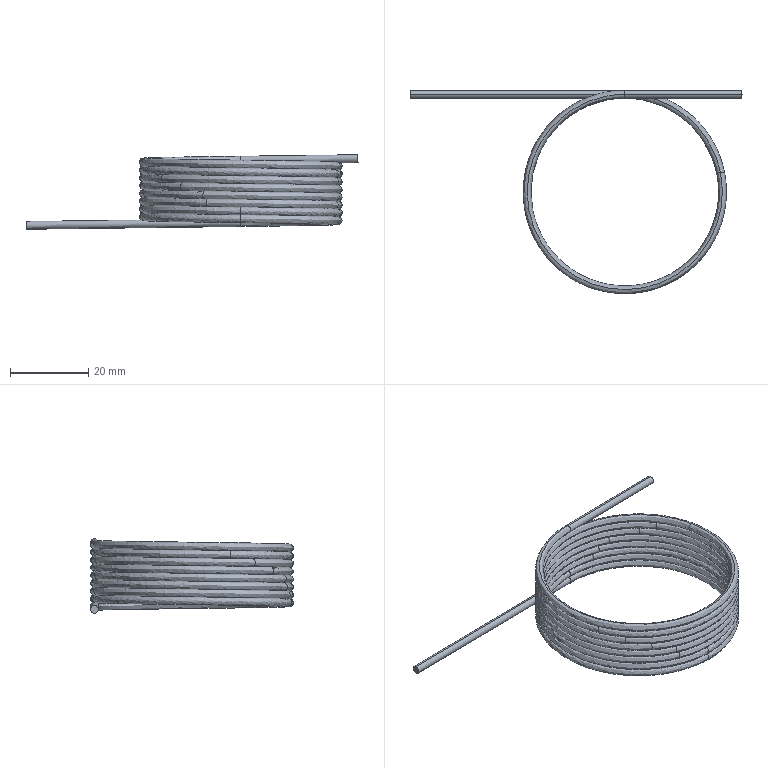Part | STEP file | 2.5 capillary tube | 3 solids | 40 faces | box 85.019 x 52 x 19.082 mm | volume 4215 mm3 | spline 30 | plane 6 | cylinder 4 | commonest cylinder face diameters 2 x4